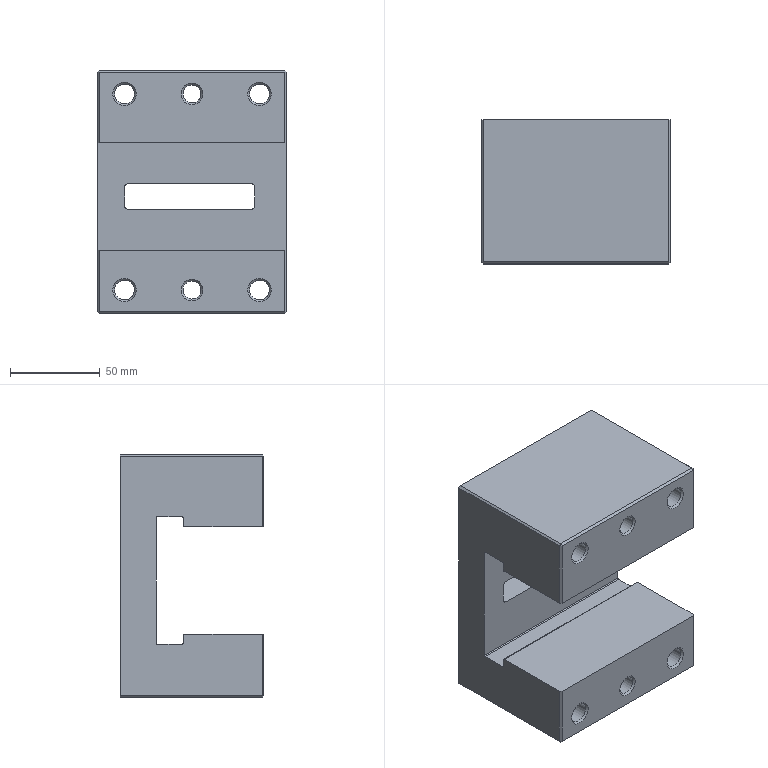Part | STEP file | solid 49 | 1 solid | 72 faces | box 105 x 80 x 135 mm | volume 660934 mm3 | plane 38 | cylinder 24 | cone 10 | commonest cylinder face diameters 1 x6 4 x4 11 x4 18 x4 5 x2 10 x2